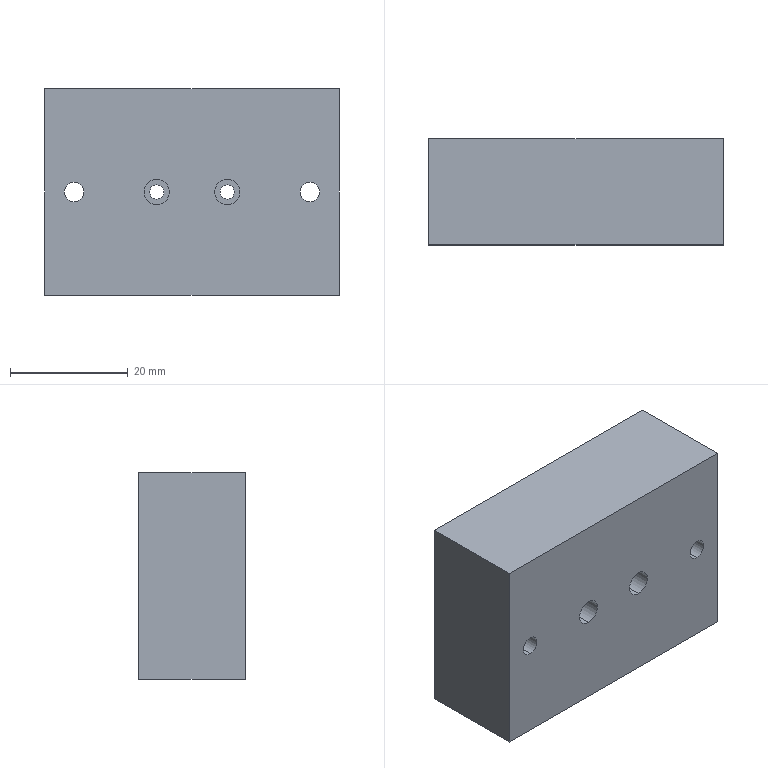Part | STEP file | Camera connecting plate | 1 solid | 24 faces | box 50 x 18 x 35 mm | volume 30828 mm3 | cylinder 12 | plane 8 | cone 4 | commonest cylinder face diameters 2.4 x4 3.3 x4 4.3 x4